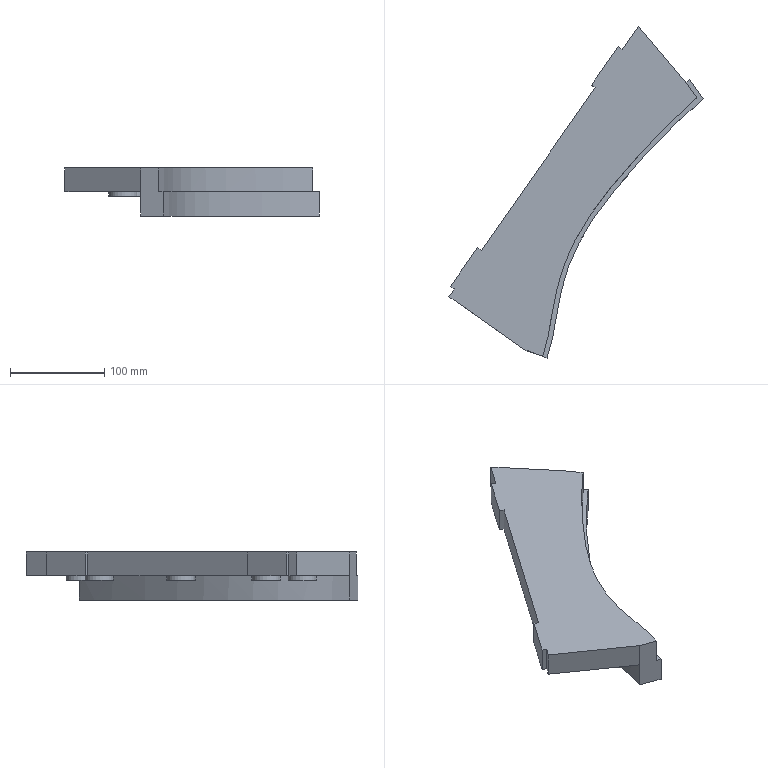Part | NX | features solid 2 | 1 solid | 31 faces | box 269.447 x 351.962 x 51 mm | volume 972041 mm3 | plane 23 | cylinder 5 | spline 3 | commonest cylinder face diameters 30 x5
STEP:
#1=CARTESIAN_POINT('',(-705.315,422.817,20.));
#2=VERTEX_POINT('',#1);
#3=CARTESIAN_POINT('',(-688.108,447.392,20.));
#4=VERTEX_POINT('',#3);
#5=CARTESIAN_POINT('',(-905.716,136.616,20.));
#6=DIRECTION('',(0.5736,0.8192,0.));
#7=VECTOR('',#6,1000.);
#8=LINE('',#5,#7);
#9=EDGE_CURVE('',#2,#4,#8,.T.);
#10=ORIENTED_EDGE('',*,*,#9,.T.);
#11=CARTESIAN_POINT('',(-637.845,387.49,20.));
#12=VERTEX_POINT('',#11);
#13=CARTESIAN_POINT('',(-624.41,371.479,20.));
#14=DIRECTION('',(-0.6428,0.766,0.));
#15=VECTOR('',#14,1000.);
#16=LINE('',#13,#15);
#17=EDGE_CURVE('',#12,#4,#16,.T.);
#18=ORIENTED_EDGE('',*,*,#17,.F.);
#19=CARTESIAN_POINT('',(-808.507,103.989,20.));
#20=VERTEX_POINT('',#19);
#21=CARTESIAN_POINT('',(-808.507,103.989,20.));
#22=CARTESIAN_POINT('',(-807.443,107.395,20.));
#23=CARTESIAN_POINT('',(-805.147,114.169,20.));
#24=CARTESIAN_POINT('',(-802.95,124.611,20.));
#25=CARTESIAN_POINT('',(-801.224,135.158,20.));
#26=CARTESIAN_POINT('',(-798.981,149.234,20.));
#27=CARTESIAN_POINT('',(-795.817,166.743,20.));
#28=CARTESIAN_POINT('',(-790.541,187.447,20.));
#29=CARTESIAN_POINT('',(-783.448,207.655,20.));
#30=CARTESIAN_POINT('',(-774.7,226.871,20.));
#31=CARTESIAN_POINT('',(-764.413,245.291,20.));
#32=CARTESIAN_POINT('',(-752.798,262.981,20.));
#33=CARTESIAN_POINT('',(-740.061,280.104,20.));
#34=CARTESIAN_POINT('',(-722.23,302.101,20.));
#35=CARTESIAN_POINT('',(-698.758,328.491,20.));
#36=CARTESIAN_POINT('',(-669.348,358.978,20.));
#37=CARTESIAN_POINT('',(-648.629,378.254,20.));
#38=CARTESIAN_POINT('',(-637.845,387.49,20.));
#39=B_SPLINE_CURVE_WITH_KNOTS('',3,(#21,#22,#23,#24,#25,#26,#27,#28,#29,#30,#31,#32,#33,#34,#35,#36,#37,#38),.UNSPECIFIED.,.F.,.F.,(4,1,1,1,1,1,1,1,1,1,1,1,1,1,1,4),(0.,0.01067,0.02134,0.03201,0.04268,0.06401,0.08535,0.1067,0.128,0.1494,0.1707,0.192,0.2134,0.2561,0.2987,0.3414),.UNSPECIFIED.);
#40=EDGE_CURVE('',#20,#12,#39,.T.);
#41=ORIENTED_EDGE('',*,*,#40,.F.);
#42=CARTESIAN_POINT('',(-889.065,160.396,20.));
#43=VERTEX_POINT('',#42);
#44=CARTESIAN_POINT('',(-845.649,129.996,20.));
#45=DIRECTION('',(-0.8192,0.5736,0.));
#46=VECTOR('',#45,1000.);
#47=LINE('',#44,#46);
#48=EDGE_CURVE('',#20,#43,#47,.T.);
#49=ORIENTED_EDGE('',*,*,#48,.T.);
#50=CARTESIAN_POINT('',(-883.329,168.587,20.));
#51=VERTEX_POINT('',#50);
#52=CARTESIAN_POINT('',(-905.716,136.616,20.));
#53=DIRECTION('',(0.5736,0.8192,0.));
#54=VECTOR('',#53,1000.);
#55=LINE('',#52,#54);
#56=EDGE_CURVE('',#43,#51,#55,.T.);
#57=ORIENTED_EDGE('',*,*,#56,.T.);
#58=CARTESIAN_POINT('',(-887.425,171.455,20.));
#59=VERTEX_POINT('',#58);
#60=CARTESIAN_POINT('',(-757.38,80.397,20.));
#61=DIRECTION('',(-0.8192,0.5736,0.));
#62=VECTOR('',#61,1000.);
#63=LINE('',#60,#62);
#64=EDGE_CURVE('',#59,#51,#63,.F.);
#65=ORIENTED_EDGE('',*,*,#64,.F.);
#66=CARTESIAN_POINT('',(-858.746,212.413,20.));
#67=VERTEX_POINT('',#66);
#68=CARTESIAN_POINT('',(-909.812,139.483,20.));
#69=DIRECTION('',(0.5736,0.8192,0.));
#70=VECTOR('',#69,1000.);
#71=LINE('',#68,#70);
#72=EDGE_CURVE('',#59,#67,#71,.T.);
#73=ORIENTED_EDGE('',*,*,#72,.T.);
#74=CARTESIAN_POINT('',(-854.65,209.545,20.));
#75=VERTEX_POINT('',#74);
#76=CARTESIAN_POINT('',(-728.701,121.354,20.));
#77=DIRECTION('',(-0.8192,0.5736,0.));
#78=VECTOR('',#77,1000.);
#79=LINE('',#76,#78);
#80=EDGE_CURVE('',#67,#75,#79,.F.);
#81=ORIENTED_EDGE('',*,*,#80,.T.);
#82=CARTESIAN_POINT('',(-733.994,381.859,20.));
#83=VERTEX_POINT('',#82);
#84=CARTESIAN_POINT('',(-905.716,136.616,20.));
#85=DIRECTION('',(0.5736,0.8192,0.));
#86=VECTOR('',#85,1000.);
#87=LINE('',#84,#86);
#88=EDGE_CURVE('',#75,#83,#87,.T.);
#89=ORIENTED_EDGE('',*,*,#88,.T.);
#90=CARTESIAN_POINT('',(-738.09,384.727,20.));
#91=VERTEX_POINT('',#90);
#92=CARTESIAN_POINT('',(-738.09,384.727,20.));
#93=DIRECTION('',(0.8192,-0.5736,0.));
#94=VECTOR('',#93,1000.);
#95=LINE('',#92,#94);
#96=EDGE_CURVE('',#91,#83,#95,.T.);
#97=ORIENTED_EDGE('',*,*,#96,.F.);
#98=CARTESIAN_POINT('',(-709.411,425.685,20.));
#99=VERTEX_POINT('',#98);
#100=CARTESIAN_POINT('',(-749.005,369.138,20.));
#101=DIRECTION('',(0.5736,0.8192,0.));
#102=VECTOR('',#101,1000.);
#103=LINE('',#100,#102);
#104=EDGE_CURVE('',#91,#99,#103,.T.);
#105=ORIENTED_EDGE('',*,*,#104,.T.);
#106=CARTESIAN_POINT('',(-709.411,425.685,20.));
#107=DIRECTION('',(0.8192,-0.5736,0.));
#108=VECTOR('',#107,1000.);
#109=LINE('',#106,#108);
#110=EDGE_CURVE('',#99,#2,#109,.T.);
#111=ORIENTED_EDGE('',*,*,#110,.T.);
#112=EDGE_LOOP('',(#10,#18,#41,#49,#57,#65,#73,#81,#89,#97,#105,#111));
#113=FACE_BOUND('',#112,.T.);
#114=CARTESIAN_POINT('',(-814.708,161.863,20.));
#115=VERTEX_POINT('',#114);
#116=CARTESIAN_POINT('',(-827.698,154.363,20.));
#117=DIRECTION('',(0.,0.,-1.));
#118=DIRECTION('',(0.866,0.5,0.));
#119=AXIS2_PLACEMENT_3D('',#116,#117,#118);
#120=CIRCLE('',#119,15.);
#121=EDGE_CURVE('',#115,#115,#120,.T.);
#122=ORIENTED_EDGE('',*,*,#121,.F.);
#123=EDGE_LOOP('',(#122));
#124=FACE_BOUND('',#123,.T.);
#125=CARTESIAN_POINT('',(-662.172,397.305,20.));
#126=VERTEX_POINT('',#125);
#127=CARTESIAN_POINT('',(-675.163,389.805,20.));
#128=DIRECTION('',(0.,0.,-1.));
#129=DIRECTION('',(0.866,0.5,0.));
#130=AXIS2_PLACEMENT_3D('',#127,#128,#129);
#131=CIRCLE('',#130,15.);
#132=EDGE_CURVE('',#126,#126,#131,.T.);
#133=ORIENTED_EDGE('',*,*,#132,.F.);
#134=EDGE_LOOP('',(#133));
#135=FACE_BOUND('',#134,.T.);
#136=CARTESIAN_POINT('',(-696.814,377.305,20.));
#137=VERTEX_POINT('',#136);
#138=CARTESIAN_POINT('',(-709.804,369.805,20.));
#139=DIRECTION('',(0.,0.,-1.));
#140=DIRECTION('',(0.866,0.5,0.));
#141=AXIS2_PLACEMENT_3D('',#138,#139,#140);
#142=CIRCLE('',#141,15.);
#143=EDGE_CURVE('',#137,#137,#142,.T.);
#144=ORIENTED_EDGE('',*,*,#143,.F.);
#145=EDGE_LOOP('',(#144));
#146=FACE_BOUND('',#145,.T.);
#147=CARTESIAN_POINT('',(-808.057,200.344,20.));
#148=VERTEX_POINT('',#147);
#149=CARTESIAN_POINT('',(-821.047,192.844,20.));
#150=DIRECTION('',(0.,0.,-1.));
#151=DIRECTION('',(0.866,0.5,0.));
#152=AXIS2_PLACEMENT_3D('',#149,#150,#151);
#153=CIRCLE('',#152,15.);
#154=EDGE_CURVE('',#148,#148,#153,.T.);
#155=ORIENTED_EDGE('',*,*,#154,.F.);
#156=EDGE_LOOP('',(#155));
#157=FACE_BOUND('',#156,.T.);
#158=CARTESIAN_POINT('',(-759.935,290.655,20.));
#159=VERTEX_POINT('',#158);
#160=CARTESIAN_POINT('',(-772.926,283.155,20.));
#161=DIRECTION('',(0.,0.,-1.));
#162=DIRECTION('',(0.866,0.5,0.));
#163=AXIS2_PLACEMENT_3D('',#160,#161,#162);
#164=CIRCLE('',#163,15.);
#165=EDGE_CURVE('',#159,#159,#164,.T.);
#166=ORIENTED_EDGE('',*,*,#165,.F.);
#167=EDGE_LOOP('',(#166));
#168=FACE_BOUND('',#167,.T.);
#169=CARTESIAN_POINT('',(-561.977,359.461,20.));
#170=DIRECTION('',(0.,0.,-1.));
#171=DIRECTION('',(-1.,0.,0.));
#172=AXIS2_PLACEMENT_3D('',#169,#170,#171);
#173=PLANE('',#172);
#174=ADVANCED_FACE('',(#113,#124,#135,#146,#157,#168),#173,.T.);
#175=CARTESIAN_POINT('',(-626.316,371.025,45.));
#176=VERTEX_POINT('',#175);
#177=CARTESIAN_POINT('',(-637.845,387.49,45.));
#178=VERTEX_POINT('',#177);
#179=CARTESIAN_POINT('',(-601.969,336.255,45.));
#180=DIRECTION('',(-0.5736,0.8192,0.));
#181=VECTOR('',#180,1000.);
#182=LINE('',#179,#181);
#183=EDGE_CURVE('',#176,#178,#182,.T.);
#184=ORIENTED_EDGE('',*,*,#183,.F.);
#185=CARTESIAN_POINT('',(-626.316,371.025,20.));
#186=VERTEX_POINT('',#185);
#187=CARTESIAN_POINT('',(-626.316,371.025,29.5));
#188=DIRECTION('',(0.,0.,1.));
#189=VECTOR('',#188,1000.);
#190=LINE('',#187,#189);
#191=EDGE_CURVE('',#176,#186,#190,.F.);
#192=ORIENTED_EDGE('',*,*,#191,.T.);
#193=CARTESIAN_POINT('',(-601.969,336.255,20.));
#194=DIRECTION('',(0.5736,-0.8192,0.));
#195=VECTOR('',#194,1000.);
#196=LINE('',#193,#195);
#197=EDGE_CURVE('',#186,#12,#196,.F.);
#198=ORIENTED_EDGE('',*,*,#197,.T.);
#199=CARTESIAN_POINT('',(-637.845,387.49,20.));
#200=DIRECTION('',(0.,0.,1.));
#201=VECTOR('',#200,1000.);
#202=LINE('',#199,#201);
#203=EDGE_CURVE('',#12,#178,#202,.T.);
#204=ORIENTED_EDGE('',*,*,#203,.T.);
#205=EDGE_LOOP('',(#184,#192,#198,#204));
#206=FACE_BOUND('',#205,.T.);
#207=CARTESIAN_POINT('',(-601.969,336.255,45.));
#208=DIRECTION('',(-0.8192,-0.5736,0.));
#209=DIRECTION('',(0.5736,-0.8192,0.));
#210=AXIS2_PLACEMENT_3D('',#207,#208,#209);
#211=PLANE('',#210);
#212=ADVANCED_FACE('',(#206),#211,.F.);
#213=CARTESIAN_POINT('',(-619.617,370.176,20.));
#214=VERTEX_POINT('',#213);
#215=CARTESIAN_POINT('',(-619.617,370.176,-6.));
#216=VERTEX_POINT('',#215);
#217=CARTESIAN_POINT('',(-619.617,370.176,45.));
#218=DIRECTION('',(0.,0.,-1.));
#219=VECTOR('',#218,1000.);
#220=LINE('',#217,#219);
#221=EDGE_CURVE('',#214,#216,#220,.T.);
#222=ORIENTED_EDGE('',*,*,#221,.F.);
#223=CARTESIAN_POINT('',(-784.99,95.429,20.));
#224=VERTEX_POINT('',#223);
#225=CARTESIAN_POINT('',(-619.617,370.176,20.));
#226=CARTESIAN_POINT('',(-620.758,369.209,20.));
#227=CARTESIAN_POINT('',(-633.301,358.48,20.));
#228=CARTESIAN_POINT('',(-656.232,336.831,20.));
#229=CARTESIAN_POINT('',(-687.219,304.143,20.));
#230=CARTESIAN_POINT('',(-716.713,270.098,20.));
#231=CARTESIAN_POINT('',(-738.935,239.768,20.));
#232=CARTESIAN_POINT('',(-753.526,213.482,20.));
#233=CARTESIAN_POINT('',(-762.494,192.807,20.));
#234=CARTESIAN_POINT('',(-769.153,171.263,20.));
#235=CARTESIAN_POINT('',(-773.765,149.208,20.));
#236=CARTESIAN_POINT('',(-776.568,130.653,20.));
#237=CARTESIAN_POINT('',(-778.83,117.715,20.));
#238=CARTESIAN_POINT('',(-780.455,110.384,20.));
#239=CARTESIAN_POINT('',(-781.918,105.166,20.));
#240=CARTESIAN_POINT('',(-783.499,100.202,20.));
#241=CARTESIAN_POINT('',(-784.493,97.02,20.));
#242=CARTESIAN_POINT('',(-784.99,95.429,20.));
#243=B_SPLINE_CURVE_WITH_KNOTS('',3,(#225,#226,#227,#228,#229,#230,#231,#232,#233,#234,#235,#236,#237,#238,#239,#240,#241,#242),.UNSPECIFIED.,.F.,.F.,(4,1,1,1,1,1,1,1,1,1,1,1,1,1,1,4),(0.,0.0136,0.1502,0.2868,0.4233,0.5599,0.6282,0.6965,0.7648,0.8331,0.9014,0.9355,0.9526,0.9697,0.9848,1.),.UNSPECIFIED.);
#244=EDGE_CURVE('',#224,#214,#243,.F.);
#245=ORIENTED_EDGE('',*,*,#244,.F.);
#246=CARTESIAN_POINT('',(-784.99,95.429,-6.));
#247=VERTEX_POINT('',#246);
#248=CARTESIAN_POINT('',(-784.99,95.429,45.));
#249=DIRECTION('',(0.,0.,-1.));
#250=VECTOR('',#249,1000.);
#251=LINE('',#248,#250);
#252=EDGE_CURVE('',#224,#247,#251,.T.);
#253=ORIENTED_EDGE('',*,*,#252,.T.);
#254=CARTESIAN_POINT('',(-619.617,370.176,-6.));
#255=CARTESIAN_POINT('',(-620.758,369.209,-6.));
#256=CARTESIAN_POINT('',(-633.301,358.48,-6.));
#257=CARTESIAN_POINT('',(-656.232,336.831,-6.));
#258=CARTESIAN_POINT('',(-687.219,304.143,-6.));
#259=CARTESIAN_POINT('',(-716.713,270.098,-6.));
#260=CARTESIAN_POINT('',(-738.935,239.768,-6.));
#261=CARTESIAN_POINT('',(-753.526,213.482,-6.));
#262=CARTESIAN_POINT('',(-762.494,192.807,-6.));
#263=CARTESIAN_POINT('',(-769.153,171.263,-6.));
#264=CARTESIAN_POINT('',(-773.765,149.208,-6.));
#265=CARTESIAN_POINT('',(-776.568,130.653,-6.));
#266=CARTESIAN_POINT('',(-778.83,117.715,-6.));
#267=CARTESIAN_POINT('',(-780.455,110.384,-6.));
#268=CARTESIAN_POINT('',(-781.918,105.166,-6.));
#269=CARTESIAN_POINT('',(-783.499,100.202,-6.));
#270=CARTESIAN_POINT('',(-784.493,97.02,-6.));
#271=CARTESIAN_POINT('',(-784.99,95.429,-6.));
#272=B_SPLINE_CURVE_WITH_KNOTS('',3,(#254,#255,#256,#257,#258,#259,#260,#261,#262,#263,#264,#265,#266,#267,#268,#269,#270,#271),.UNSPECIFIED.,.F.,.F.,(4,1,1,1,1,1,1,1,1,1,1,1,1,1,1,4),(0.,0.0136,0.1502,0.2868,0.4233,0.5599,0.6282,0.6965,0.7648,0.8331,0.9014,0.9355,0.9526,0.9697,0.9848,1.),.UNSPECIFIED.);
#273=EDGE_CURVE('',#216,#247,#272,.T.);
#274=ORIENTED_EDGE('',*,*,#273,.F.);
#275=EDGE_LOOP('',(#222,#245,#253,#274));
#276=FACE_BOUND('',#275,.T.);
#277=CARTESIAN_POINT('',(-619.617,370.176,20.));
#278=CARTESIAN_POINT('',(-619.617,370.176,-6.));
#279=CARTESIAN_POINT('',(-630.098,361.294,20.));
#280=CARTESIAN_POINT('',(-630.098,361.294,-6.));
#281=CARTESIAN_POINT('',(-650.295,342.645,20.));
#282=CARTESIAN_POINT('',(-650.295,342.645,-6.));
#283=CARTESIAN_POINT('',(-678.981,313.038,20.));
#284=CARTESIAN_POINT('',(-678.981,313.038,-6.));
#285=CARTESIAN_POINT('',(-706.428,282.292,20.));
#286=CARTESIAN_POINT('',(-706.428,282.292,-6.));
#287=CARTESIAN_POINT('',(-732.113,249.996,20.));
#288=CARTESIAN_POINT('',(-732.113,249.996,-6.));
#289=CARTESIAN_POINT('',(-750.21,220.698,20.));
#290=CARTESIAN_POINT('',(-750.21,220.698,-6.));
#291=CARTESIAN_POINT('',(-761.378,195.562,20.));
#292=CARTESIAN_POINT('',(-761.378,195.562,-6.));
#293=CARTESIAN_POINT('',(-767.84,175.972,20.));
#294=CARTESIAN_POINT('',(-767.84,175.972,-6.));
#295=CARTESIAN_POINT('',(-772.516,155.885,20.));
#296=CARTESIAN_POINT('',(-772.516,155.885,-6.));
#297=CARTESIAN_POINT('',(-775.302,138.936,20.));
#298=CARTESIAN_POINT('',(-775.302,138.936,-6.));
#299=CARTESIAN_POINT('',(-777.483,125.374,20.));
#300=CARTESIAN_POINT('',(-777.483,125.374,-6.));
#301=CARTESIAN_POINT('',(-779.274,115.224,20.));
#302=CARTESIAN_POINT('',(-779.274,115.224,-6.));
#303=CARTESIAN_POINT('',(-781.8,105.229,20.));
#304=CARTESIAN_POINT('',(-781.8,105.229,-6.));
#305=CARTESIAN_POINT('',(-783.966,98.707,20.));
#306=CARTESIAN_POINT('',(-783.966,98.707,-6.));
#307=CARTESIAN_POINT('',(-784.99,95.429,20.));
#308=CARTESIAN_POINT('',(-784.99,95.429,-6.));
#309=B_SPLINE_SURFACE_WITH_KNOTS('',3,1,((#277,#278),(#279,#280),(#281,#282),(#283,#284),(#285,#286),(#287,#288),(#289,#290),(#291,#292),(#293,#294),(#295,#296),(#297,#298),(#299,#300),(#301,#302),(#303,#304),(#305,#306),(#307,#308)),.SURF_OF_LINEAR_EXTRUSION.,.F.,.F.,.F.,(4,1,1,1,1,1,1,1,1,1,1,1,1,4),(2,2),(0.,0.125,0.25,0.375,0.5,0.625,0.6875,0.75,0.8125,0.875,0.9062,0.9375,0.9688,1.),(0.,1.),.UNSPECIFIED.);
#310=ADVANCED_FACE('',(#276),#309,.T.);
#311=ORIENTED_EDGE('',*,*,#17,.T.);
#312=CARTESIAN_POINT('',(-688.108,447.392,45.));
#313=VERTEX_POINT('',#312);
#314=CARTESIAN_POINT('',(-688.108,447.392,51.));
#315=DIRECTION('',(0.,0.,-1.));
#316=VECTOR('',#315,1000.);
#317=LINE('',#314,#316);
#318=EDGE_CURVE('',#313,#4,#317,.T.);
#319=ORIENTED_EDGE('',*,*,#318,.F.);
#320=CARTESIAN_POINT('',(-624.41,371.479,45.));
#321=DIRECTION('',(-0.6428,0.766,0.));
#322=VECTOR('',#321,1000.);
#323=LINE('',#320,#322);
#324=EDGE_CURVE('',#178,#313,#323,.T.);
#325=ORIENTED_EDGE('',*,*,#324,.F.);
#326=ORIENTED_EDGE('',*,*,#203,.F.);
#327=EDGE_LOOP('',(#311,#319,#325,#326));
#328=FACE_BOUND('',#327,.T.);
#329=CARTESIAN_POINT('',(-637.845,387.49,20.));
#330=DIRECTION('',(0.766,0.6428,0.));
#331=DIRECTION('',(-0.6428,0.766,0.));
#332=AXIS2_PLACEMENT_3D('',#329,#330,#331);
#333=PLANE('',#332);
#334=ADVANCED_FACE('',(#328),#333,.T.);
#335=ORIENTED_EDGE('',*,*,#191,.F.);
#336=CARTESIAN_POINT('',(-789.693,97.141,45.));
#337=VERTEX_POINT('',#336);
#338=CARTESIAN_POINT('',(-626.316,371.025,45.));
#339=CARTESIAN_POINT('',(-636.644,362.111,45.));
#340=CARTESIAN_POINT('',(-656.576,343.456,45.));
#341=CARTESIAN_POINT('',(-684.976,313.909,45.));
#342=CARTESIAN_POINT('',(-707.592,288.428,45.));
#343=CARTESIAN_POINT('',(-724.731,267.231,45.));
#344=CARTESIAN_POINT('',(-736.956,250.736,45.));
#345=CARTESIAN_POINT('',(-748.139,233.564,45.));
#346=CARTESIAN_POINT('',(-757.889,215.763,45.));
#347=CARTESIAN_POINT('',(-766.081,197.219,45.));
#348=CARTESIAN_POINT('',(-772.504,177.826,45.));
#349=CARTESIAN_POINT('',(-777.254,157.705,45.));
#350=CARTESIAN_POINT('',(-780.079,140.755,45.));
#351=CARTESIAN_POINT('',(-782.256,127.163,45.));
#352=CARTESIAN_POINT('',(-784.018,117.,45.));
#353=CARTESIAN_POINT('',(-786.48,106.988,45.));
#354=CARTESIAN_POINT('',(-788.665,100.433,45.));
#355=CARTESIAN_POINT('',(-789.693,97.141,45.));
#356=B_SPLINE_CURVE_WITH_KNOTS('',3,(#338,#339,#340,#341,#342,#343,#344,#345,#346,#347,#348,#349,#350,#351,#352,#353,#354,#355),.UNSPECIFIED.,.F.,.F.,(4,1,1,1,1,1,1,1,1,1,1,1,1,1,1,4),(1.377,1.418,1.459,1.5,1.521,1.541,1.562,1.582,1.603,1.623,1.643,1.664,1.674,1.684,1.695,1.705),.UNSPECIFIED.);
#357=EDGE_CURVE('',#176,#337,#356,.T.);
#358=ORIENTED_EDGE('',*,*,#357,.T.);
#359=CARTESIAN_POINT('',(-789.693,97.141,20.));
#360=VERTEX_POINT('',#359);
#361=CARTESIAN_POINT('',(-789.693,97.141,32.5));
#362=DIRECTION('',(0.,0.,1.));
#363=VECTOR('',#362,1000.);
#364=LINE('',#361,#363);
#365=EDGE_CURVE('',#360,#337,#364,.T.);
#366=ORIENTED_EDGE('',*,*,#365,.F.);
#367=CARTESIAN_POINT('',(-626.316,371.025,20.));
#368=CARTESIAN_POINT('',(-636.667,362.091,20.));
#369=CARTESIAN_POINT('',(-656.605,343.424,20.));
#370=CARTESIAN_POINT('',(-684.913,313.982,20.));
#371=CARTESIAN_POINT('',(-712.011,283.428,20.));
#372=CARTESIAN_POINT('',(-737.426,251.153,20.));
#373=CARTESIAN_POINT('',(-755.401,221.588,20.));
#374=CARTESIAN_POINT('',(-766.499,196.168,20.));
#375=CARTESIAN_POINT('',(-772.915,176.364,20.));
#376=CARTESIAN_POINT('',(-777.548,156.176,20.));
#377=CARTESIAN_POINT('',(-780.308,139.294,20.));
#378=CARTESIAN_POINT('',(-782.449,125.988,20.));
#379=CARTESIAN_POINT('',(-784.207,116.114,20.));
#380=CARTESIAN_POINT('',(-786.544,106.843,20.));
#381=CARTESIAN_POINT('',(-788.684,100.373,20.));
#382=CARTESIAN_POINT('',(-789.693,97.141,20.));
#383=B_SPLINE_CURVE_WITH_KNOTS('',3,(#367,#368,#369,#370,#371,#372,#373,#374,#375,#376,#377,#378,#379,#380,#381,#382),.UNSPECIFIED.,.F.,.F.,(4,1,1,1,1,1,1,1,1,1,1,1,1,4),(0.0137,0.1369,0.2601,0.3833,0.5065,0.6297,0.6913,0.7529,0.8145,0.8761,0.9069,0.9377,0.9685,0.9993),.UNSPECIFIED.);
#384=EDGE_CURVE('',#186,#360,#383,.T.);
#385=ORIENTED_EDGE('',*,*,#384,.F.);
#386=EDGE_LOOP('',(#335,#358,#366,#385));
#387=FACE_BOUND('',#386,.T.);
#388=CARTESIAN_POINT('',(-626.316,371.025,20.));
#389=CARTESIAN_POINT('',(-626.316,371.025,45.));
#390=CARTESIAN_POINT('',(-636.667,362.091,20.));
#391=CARTESIAN_POINT('',(-636.667,362.091,45.));
#392=CARTESIAN_POINT('',(-656.605,343.424,20.));
#393=CARTESIAN_POINT('',(-656.605,343.424,45.));
#394=CARTESIAN_POINT('',(-684.913,313.982,20.));
#395=CARTESIAN_POINT('',(-684.913,313.982,45.));
#396=CARTESIAN_POINT('',(-712.011,283.428,20.));
#397=CARTESIAN_POINT('',(-712.011,283.428,45.));
#398=CARTESIAN_POINT('',(-737.426,251.153,20.));
#399=CARTESIAN_POINT('',(-737.426,251.153,45.));
#400=CARTESIAN_POINT('',(-755.401,221.588,20.));
#401=CARTESIAN_POINT('',(-755.401,221.588,45.));
#402=CARTESIAN_POINT('',(-766.499,196.168,20.));
#403=CARTESIAN_POINT('',(-766.499,196.168,45.));
#404=CARTESIAN_POINT('',(-772.915,176.364,20.));
#405=CARTESIAN_POINT('',(-772.915,176.364,45.));
#406=CARTESIAN_POINT('',(-777.548,156.176,20.));
#407=CARTESIAN_POINT('',(-777.548,156.176,45.));
#408=CARTESIAN_POINT('',(-780.308,139.294,20.));
#409=CARTESIAN_POINT('',(-780.308,139.294,45.));
#410=CARTESIAN_POINT('',(-782.449,125.988,20.));
#411=CARTESIAN_POINT('',(-782.449,125.988,45.));
#412=CARTESIAN_POINT('',(-784.207,116.114,20.));
#413=CARTESIAN_POINT('',(-784.207,116.114,45.));
#414=CARTESIAN_POINT('',(-786.544,106.843,20.));
#415=CARTESIAN_POINT('',(-786.544,106.843,45.));
#416=CARTESIAN_POINT('',(-788.684,100.373,20.));
#417=CARTESIAN_POINT('',(-788.684,100.373,45.));
#418=CARTESIAN_POINT('',(-789.693,97.141,20.));
#419=CARTESIAN_POINT('',(-789.693,97.141,45.));
#420=B_SPLINE_SURFACE_WITH_KNOTS('',3,1,((#388,#389),(#390,#391),(#392,#393),(#394,#395),(#396,#397),(#398,#399),(#400,#401),(#402,#403),(#404,#405),(#406,#407),(#408,#409),(#410,#411),(#412,#413),(#414,#415),(#416,#417),(#418,#419)),.SURF_OF_LINEAR_EXTRUSION.,.F.,.F.,.F.,(4,1,1,1,1,1,1,1,1,1,1,1,1,4),(2,2),(0.0137,0.1369,0.2601,0.3833,0.5065,0.6297,0.6913,0.7529,0.8145,0.8761,0.9069,0.9377,0.9685,0.9993),(0.,1.),.UNSPECIFIED.);
#421=ADVANCED_FACE('',(#387),#420,.F.);
#422=ORIENTED_EDGE('',*,*,#324,.T.);
#423=CARTESIAN_POINT('',(-705.315,422.817,45.));
#424=VERTEX_POINT('',#423);
#425=CARTESIAN_POINT('',(-905.716,136.616,45.));
#426=DIRECTION('',(0.5736,0.8192,0.));
#427=VECTOR('',#426,1000.);
#428=LINE('',#425,#427);
#429=EDGE_CURVE('',#424,#313,#428,.T.);
#430=ORIENTED_EDGE('',*,*,#429,.F.);
#431=CARTESIAN_POINT('',(-709.411,425.685,45.));
#432=VERTEX_POINT('',#431);
#433=CARTESIAN_POINT('',(-661.9,392.417,45.));
#434=DIRECTION('',(0.8192,-0.5736,0.));
#435=VECTOR('',#434,1000.);
#436=LINE('',#433,#435);
#437=EDGE_CURVE('',#432,#424,#436,.T.);
#438=ORIENTED_EDGE('',*,*,#437,.F.);
#439=CARTESIAN_POINT('',(-738.09,384.727,45.));
#440=VERTEX_POINT('',#439);
#441=CARTESIAN_POINT('',(-749.005,369.138,45.));
#442=DIRECTION('',(0.5736,0.8192,0.));
#443=VECTOR('',#442,1000.);
#444=LINE('',#441,#443);
#445=EDGE_CURVE('',#440,#432,#444,.T.);
#446=ORIENTED_EDGE('',*,*,#445,.F.);
#447=CARTESIAN_POINT('',(-733.994,381.859,45.));
#448=VERTEX_POINT('',#447);
#449=CARTESIAN_POINT('',(-690.579,351.459,45.));
#450=DIRECTION('',(0.8192,-0.5736,0.));
#451=VECTOR('',#450,1000.);
#452=LINE('',#449,#451);
#453=EDGE_CURVE('',#440,#448,#452,.T.);
#454=ORIENTED_EDGE('',*,*,#453,.T.);
#455=CARTESIAN_POINT('',(-854.65,209.545,45.));
#456=VERTEX_POINT('',#455);
#457=CARTESIAN_POINT('',(-905.716,136.616,45.));
#458=DIRECTION('',(0.5736,0.8192,0.));
#459=VECTOR('',#458,1000.);
#460=LINE('',#457,#459);
#461=EDGE_CURVE('',#456,#448,#460,.T.);
#462=ORIENTED_EDGE('',*,*,#461,.F.);
#463=CARTESIAN_POINT('',(-858.746,212.413,45.));
#464=VERTEX_POINT('',#463);
#465=CARTESIAN_POINT('',(-811.235,179.145,45.));
#466=DIRECTION('',(0.8192,-0.5736,0.));
#467=VECTOR('',#466,1000.);
#468=LINE('',#465,#467);
#469=EDGE_CURVE('',#464,#456,#468,.T.);
#470=ORIENTED_EDGE('',*,*,#469,.F.);
#471=CARTESIAN_POINT('',(-887.425,171.455,45.));
#472=VERTEX_POINT('',#471);
#473=CARTESIAN_POINT('',(-909.812,139.483,45.));
#474=DIRECTION('',(0.5736,0.8192,0.));
#475=VECTOR('',#474,1000.);
#476=LINE('',#473,#475);
#477=EDGE_CURVE('',#472,#464,#476,.T.);
#478=ORIENTED_EDGE('',*,*,#477,.F.);
#479=CARTESIAN_POINT('',(-883.329,168.587,45.));
#480=VERTEX_POINT('',#479);
#481=CARTESIAN_POINT('',(-839.913,138.187,45.));
#482=DIRECTION('',(0.8192,-0.5736,0.));
#483=VECTOR('',#482,1000.);
#484=LINE('',#481,#483);
#485=EDGE_CURVE('',#472,#480,#484,.T.);
#486=ORIENTED_EDGE('',*,*,#485,.T.);
#487=CARTESIAN_POINT('',(-889.065,160.396,45.));
#488=VERTEX_POINT('',#487);
#489=CARTESIAN_POINT('',(-905.716,136.616,45.));
#490=DIRECTION('',(0.5736,0.8192,0.));
#491=VECTOR('',#490,1000.);
#492=LINE('',#489,#491);
#493=EDGE_CURVE('',#488,#480,#492,.T.);
#494=ORIENTED_EDGE('',*,*,#493,.F.);
#495=CARTESIAN_POINT('',(-808.507,103.989,45.));
#496=VERTEX_POINT('',#495);
#497=CARTESIAN_POINT('',(-845.649,129.996,45.));
#498=DIRECTION('',(-0.8192,0.5736,0.));
#499=VECTOR('',#498,1000.);
#500=LINE('',#497,#499);
#501=EDGE_CURVE('',#496,#488,#500,.T.);
#502=ORIENTED_EDGE('',*,*,#501,.F.);
#503=CARTESIAN_POINT('',(-808.507,103.989,45.));
#504=DIRECTION('',(-0.9397,0.342,0.));
#505=VECTOR('',#504,1000.);
#506=LINE('',#503,#505);
#507=EDGE_CURVE('',#337,#496,#506,.T.);
#508=ORIENTED_EDGE('',*,*,#507,.F.);
#509=ORIENTED_EDGE('',*,*,#357,.F.);
#510=ORIENTED_EDGE('',*,*,#183,.T.);
#511=EDGE_LOOP('',(#422,#430,#438,#446,#454,#462,#470,#478,#486,#494,#502,#508,#509,#510));
#512=FACE_BOUND('',#511,.T.);
#513=CARTESIAN_POINT('',(-750.849,265.384,45.));
#514=DIRECTION('',(0.,0.,1.));
#515=DIRECTION('',(1.,0.,0.));
#516=AXIS2_PLACEMENT_3D('',#513,#514,#515);
#517=PLANE('',#516);
#518=ADVANCED_FACE('',(#512),#517,.T.);
#519=ORIENTED_EDGE('',*,*,#384,.T.);
#520=CARTESIAN_POINT('',(-808.507,103.989,20.));
#521=DIRECTION('',(-0.9397,0.342,0.));
#522=VECTOR('',#521,1000.);
#523=LINE('',#520,#522);
#524=EDGE_CURVE('',#224,#360,#523,.T.);
#525=ORIENTED_EDGE('',*,*,#524,.F.);
#526=ORIENTED_EDGE('',*,*,#244,.T.);
#527=CARTESIAN_POINT('',(-634.015,390.737,20.));
#528=VERTEX_POINT('',#527);
#529=CARTESIAN_POINT('',(-619.617,370.176,20.));
#530=DIRECTION('',(0.5736,-0.8192,0.));
#531=VECTOR('',#530,1000.);
#532=LINE('',#529,#531);
#533=EDGE_CURVE('',#528,#214,#532,.T.);
#534=ORIENTED_EDGE('',*,*,#533,.F.);
#535=CARTESIAN_POINT('',(-808.507,103.989,20.));
#536=CARTESIAN_POINT('',(-808.333,104.544,20.));
#537=CARTESIAN_POINT('',(-807.867,106.034,20.));
#538=CARTESIAN_POINT('',(-806.776,109.497,20.));
#539=CARTESIAN_POINT('',(-805.771,112.695,20.));
#540=CARTESIAN_POINT('',(-804.96,115.635,20.));
#541=CARTESIAN_POINT('',(-804.266,118.437,20.));
#542=CARTESIAN_POINT('',(-803.072,124.11,20.));
#543=CARTESIAN_POINT('',(-801.552,133.064,20.));
#544=CARTESIAN_POINT('',(-799.74,144.503,20.));
#545=CARTESIAN_POINT('',(-797.693,156.521,20.));
#546=CARTESIAN_POINT('',(-794.374,172.832,20.));
#547=CARTESIAN_POINT('',(-788.796,193.527,20.));
#548=CARTESIAN_POINT('',(-779.275,217.734,20.));
#549=CARTESIAN_POINT('',(-767.447,240.431,20.));
#550=CARTESIAN_POINT('',(-753.831,261.642,20.));
#551=CARTESIAN_POINT('',(-739.131,281.358,20.));
#552=CARTESIAN_POINT('',(-723.87,299.991,20.));
#553=CARTESIAN_POINT('',(-702.884,323.901,20.));
#554=CARTESIAN_POINT('',(-675.814,352.632,20.));
#555=CARTESIAN_POINT('',(-650.572,376.631,20.));
#556=CARTESIAN_POINT('',(-636.144,388.949,20.));
#557=CARTESIAN_POINT('',(-634.015,390.737,20.));
#558=B_SPLINE_CURVE_WITH_KNOTS('',3,(#535,#536,#537,#538,#539,#540,#541,#542,#543,#544,#545,#546,#547,#548,#549,#550,#551,#552,#553,#554,#555,#556,#557),.UNSPECIFIED.,.F.,.F.,(4,1,1,1,1,1,1,1,1,1,1,1,1,1,1,1,1,1,1,1,4),(0.,0.005252,0.014,0.03149,0.04023,0.04898,0.06647,0.1015,0.1364,0.1714,0.2064,0.2764,0.3463,0.4163,0.4863,0.5562,0.6262,0.6962,0.8361,0.976,1.),.UNSPECIFIED.);
#559=EDGE_CURVE('',#528,#12,#558,.F.);
#560=ORIENTED_EDGE('',*,*,#559,.T.);
#561=ORIENTED_EDGE('',*,*,#197,.F.);
#562=EDGE_LOOP('',(#519,#525,#526,#534,#560,#561));
#563=FACE_BOUND('',#562,.T.);
#564=CARTESIAN_POINT('',(-619.617,370.176,20.));
#565=DIRECTION('',(0.,0.,-1.));
#566=DIRECTION('',(-1.,0.,0.));
#567=AXIS2_PLACEMENT_3D('',#564,#565,#566);
#568=PLANE('',#567);
#569=ADVANCED_FACE('',(#563),#568,.F.);
#570=ORIENTED_EDGE('',*,*,#501,.T.);
#571=CARTESIAN_POINT('',(-889.065,160.396,51.));
#572=DIRECTION('',(0.,0.,-1.));
#573=VECTOR('',#572,1000.);
#574=LINE('',#571,#573);
#575=EDGE_CURVE('',#488,#43,#574,.T.);
#576=ORIENTED_EDGE('',*,*,#575,.T.);
#577=ORIENTED_EDGE('',*,*,#48,.F.);
#578=CARTESIAN_POINT('',(-808.507,103.989,51.));
#579=DIRECTION('',(0.,0.,1.));
#580=VECTOR('',#579,1000.);
#581=LINE('',#578,#580);
#582=EDGE_CURVE('',#20,#496,#581,.T.);
#583=ORIENTED_EDGE('',*,*,#582,.T.);
#584=EDGE_LOOP('',(#570,#576,#577,#583));
#585=FACE_BOUND('',#584,.T.);
#586=CARTESIAN_POINT('',(-808.507,103.989,20.));
#587=DIRECTION('',(0.5736,0.8192,0.));
#588=DIRECTION('',(-0.8192,0.5736,0.));
#589=AXIS2_PLACEMENT_3D('',#586,#587,#588);
#590=PLANE('',#589);
#591=ADVANCED_FACE('',(#585),#590,.F.);
#592=ORIENTED_EDGE('',*,*,#582,.F.);
#593=CARTESIAN_POINT('',(-808.507,103.989,-6.));
#594=VERTEX_POINT('',#593);
#595=CARTESIAN_POINT('',(-808.507,103.989,45.));
#596=DIRECTION('',(0.,0.,-1.));
#597=VECTOR('',#596,1000.);
#598=LINE('',#595,#597);
#599=EDGE_CURVE('',#20,#594,#598,.T.);
#600=ORIENTED_EDGE('',*,*,#599,.T.);
#601=CARTESIAN_POINT('',(-808.507,103.989,-6.));
#602=DIRECTION('',(0.9397,-0.342,0.));
#603=VECTOR('',#602,1000.);
#604=LINE('',#601,#603);
#605=EDGE_CURVE('',#594,#247,#604,.T.);
#606=ORIENTED_EDGE('',*,*,#605,.T.);
#607=ORIENTED_EDGE('',*,*,#252,.F.);
#608=ORIENTED_EDGE('',*,*,#524,.T.);
#609=ORIENTED_EDGE('',*,*,#365,.T.);
#610=ORIENTED_EDGE('',*,*,#507,.T.);
#611=EDGE_LOOP('',(#592,#600,#606,#607,#608,#609,#610));
#612=FACE_BOUND('',#611,.T.);
#613=CARTESIAN_POINT('',(-808.507,103.989,51.));
#614=DIRECTION('',(-0.342,-0.9397,0.));
#615=DIRECTION('',(0.9397,-0.342,0.));
#616=AXIS2_PLACEMENT_3D('',#613,#614,#615);
#617=PLANE('',#616);
#618=ADVANCED_FACE('',(#612),#617,.T.);
#619=ORIENTED_EDGE('',*,*,#599,.F.);
#620=ORIENTED_EDGE('',*,*,#40,.T.);
#621=ORIENTED_EDGE('',*,*,#559,.F.);
#622=CARTESIAN_POINT('',(-634.015,390.737,-6.));
#623=VERTEX_POINT('',#622);
#624=CARTESIAN_POINT('',(-634.015,390.737,45.));
#625=DIRECTION('',(0.,0.,-1.));
#626=VECTOR('',#625,1000.);
#627=LINE('',#624,#626);
#628=EDGE_CURVE('',#528,#623,#627,.T.);
#629=ORIENTED_EDGE('',*,*,#628,.T.);
#630=CARTESIAN_POINT('',(-808.507,103.989,-6.));
#631=CARTESIAN_POINT('',(-808.333,104.544,-6.));
#632=CARTESIAN_POINT('',(-807.867,106.034,-6.));
#633=CARTESIAN_POINT('',(-806.776,109.497,-6.));
#634=CARTESIAN_POINT('',(-805.771,112.695,-6.));
#635=CARTESIAN_POINT('',(-804.96,115.635,-6.));
#636=CARTESIAN_POINT('',(-804.266,118.437,-6.));
#637=CARTESIAN_POINT('',(-803.072,124.11,-6.));
#638=CARTESIAN_POINT('',(-801.552,133.064,-6.));
#639=CARTESIAN_POINT('',(-799.74,144.503,-6.));
#640=CARTESIAN_POINT('',(-797.693,156.521,-6.));
#641=CARTESIAN_POINT('',(-794.374,172.832,-6.));
#642=CARTESIAN_POINT('',(-788.796,193.527,-6.));
#643=CARTESIAN_POINT('',(-779.275,217.734,-6.));
#644=CARTESIAN_POINT('',(-767.447,240.431,-6.));
#645=CARTESIAN_POINT('',(-753.831,261.642,-6.));
#646=CARTESIAN_POINT('',(-739.131,281.358,-6.));
#647=CARTESIAN_POINT('',(-723.87,299.991,-6.));
#648=CARTESIAN_POINT('',(-702.884,323.901,-6.));
#649=CARTESIAN_POINT('',(-675.814,352.632,-6.));
#650=CARTESIAN_POINT('',(-650.572,376.631,-6.));
#651=CARTESIAN_POINT('',(-636.144,388.949,-6.));
#652=CARTESIAN_POINT('',(-634.015,390.737,-6.));
#653=B_SPLINE_CURVE_WITH_KNOTS('',3,(#630,#631,#632,#633,#634,#635,#636,#637,#638,#639,#640,#641,#642,#643,#644,#645,#646,#647,#648,#649,#650,#651,#652),.UNSPECIFIED.,.F.,.F.,(4,1,1,1,1,1,1,1,1,1,1,1,1,1,1,1,1,1,1,1,4),(0.,0.005252,0.014,0.03149,0.04023,0.04898,0.06647,0.1015,0.1364,0.1714,0.2064,0.2764,0.3463,0.4163,0.4863,0.5562,0.6262,0.6962,0.8361,0.976,1.),.UNSPECIFIED.);
#654=EDGE_CURVE('',#594,#623,#653,.T.);
#655=ORIENTED_EDGE('',*,*,#654,.F.);
#656=EDGE_LOOP('',(#619,#620,#621,#629,#655));
#657=FACE_BOUND('',#656,.T.);
#658=CARTESIAN_POINT('',(-808.507,103.989,20.));
#659=CARTESIAN_POINT('',(-808.507,103.989,-6.));
#660=CARTESIAN_POINT('',(-807.991,105.642,20.));
#661=CARTESIAN_POINT('',(-807.991,105.642,-6.));
#662=CARTESIAN_POINT('',(-806.886,109.14,20.));
#663=CARTESIAN_POINT('',(-806.886,109.14,-6.));
#664=CARTESIAN_POINT('',(-805.545,113.441,20.));
#665=CARTESIAN_POINT('',(-805.545,113.441,-6.));
#666=CARTESIAN_POINT('',(-804.551,117.174,20.));
#667=CARTESIAN_POINT('',(-804.551,117.174,-6.));
#668=CARTESIAN_POINT('',(-803.645,121.342,20.));
#669=CARTESIAN_POINT('',(-803.645,121.342,-6.));
#670=CARTESIAN_POINT('',(-802.775,125.938,20.));
#671=CARTESIAN_POINT('',(-802.775,125.938,-6.));
#672=CARTESIAN_POINT('',(-801.679,132.325,20.));
#673=CARTESIAN_POINT('',(-801.679,132.325,-6.));
#674=CARTESIAN_POINT('',(-799.808,144.073,20.));
#675=CARTESIAN_POINT('',(-799.808,144.073,-6.));
#676=CARTESIAN_POINT('',(-796.802,162.068,20.));
#677=CARTESIAN_POINT('',(-796.802,162.068,-6.));
#678=CARTESIAN_POINT('',(-791.545,184.171,20.));
#679=CARTESIAN_POINT('',(-791.545,184.171,-6.));
#680=CARTESIAN_POINT('',(-784.119,206.139,20.));
#681=CARTESIAN_POINT('',(-784.119,206.139,-6.));
#682=CARTESIAN_POINT('',(-771.443,234.184,20.));
#683=CARTESIAN_POINT('',(-771.443,234.184,-6.));
#684=CARTESIAN_POINT('',(-751.344,266.147,20.));
#685=CARTESIAN_POINT('',(-751.344,266.147,-6.));
#686=CARTESIAN_POINT('',(-724.258,299.926,20.));
#687=CARTESIAN_POINT('',(-724.258,299.926,-6.));
#688=CARTESIAN_POINT('',(-695.94,331.532,20.));
#689=CARTESIAN_POINT('',(-695.94,331.532,-6.));
#690=CARTESIAN_POINT('',(-666.316,361.972,20.));
#691=CARTESIAN_POINT('',(-666.316,361.972,-6.));
#692=CARTESIAN_POINT('',(-645.109,381.421,20.));
#693=CARTESIAN_POINT('',(-645.109,381.421,-6.));
#694=CARTESIAN_POINT('',(-634.015,390.737,20.));
#695=CARTESIAN_POINT('',(-634.015,390.737,-6.));
#696=B_SPLINE_SURFACE_WITH_KNOTS('',3,1,((#658,#659),(#660,#661),(#662,#663),(#664,#665),(#666,#667),(#668,#669),(#670,#671),(#672,#673),(#674,#675),(#676,#677),(#678,#679),(#680,#681),(#682,#683),(#684,#685),(#686,#687),(#688,#689),(#690,#691),(#692,#693),(#694,#695)),.SURF_OF_LINEAR_EXTRUSION.,.F.,.F.,.F.,(4,1,1,1,1,1,1,1,1,1,1,1,1,1,1,1,4),(2,2),(0.,0.01562,0.03125,0.04688,0.0625,0.07812,0.09375,0.125,0.1875,0.25,0.3125,0.375,0.5,0.625,0.75,0.875,1.),(0.,1.),.UNSPECIFIED.);
#697=ADVANCED_FACE('',(#657),#696,.T.);
#698=CARTESIAN_POINT('',(-619.617,370.176,-6.));
#699=DIRECTION('',(-0.5736,0.8192,0.));
#700=VECTOR('',#699,1000.);
#701=LINE('',#698,#700);
#702=EDGE_CURVE('',#216,#623,#701,.T.);
#703=ORIENTED_EDGE('',*,*,#702,.T.);
#704=ORIENTED_EDGE('',*,*,#628,.F.);
#705=ORIENTED_EDGE('',*,*,#533,.T.);
#706=ORIENTED_EDGE('',*,*,#221,.T.);
#707=EDGE_LOOP('',(#703,#704,#705,#706));
#708=FACE_BOUND('',#707,.T.);
#709=CARTESIAN_POINT('',(-634.015,390.737,51.));
#710=DIRECTION('',(-0.8192,-0.5736,0.));
#711=DIRECTION('',(0.5736,-0.8192,0.));
#712=AXIS2_PLACEMENT_3D('',#709,#710,#711);
#713=PLANE('',#712);
#714=ADVANCED_FACE('',(#708),#713,.F.);
#715=ORIENTED_EDGE('',*,*,#654,.T.);
#716=ORIENTED_EDGE('',*,*,#702,.F.);
#717=ORIENTED_EDGE('',*,*,#273,.T.);
#718=ORIENTED_EDGE('',*,*,#605,.F.);
#719=EDGE_LOOP('',(#715,#716,#717,#718));
#720=FACE_BOUND('',#719,.T.);
#721=CARTESIAN_POINT('',(-750.849,265.384,-6.));
#722=DIRECTION('',(0.,0.,1.));
#723=DIRECTION('',(1.,0.,0.));
#724=AXIS2_PLACEMENT_3D('',#721,#722,#723);
#725=PLANE('',#724);
#726=ADVANCED_FACE('',(#720),#725,.F.);
#727=ORIENTED_EDGE('',*,*,#88,.F.);
#728=CARTESIAN_POINT('',(-854.65,209.545,51.));
#729=DIRECTION('',(0.,0.,-1.));
#730=VECTOR('',#729,1000.);
#731=LINE('',#728,#730);
#732=EDGE_CURVE('',#456,#75,#731,.T.);
#733=ORIENTED_EDGE('',*,*,#732,.F.);
#734=ORIENTED_EDGE('',*,*,#461,.T.);
#735=CARTESIAN_POINT('',(-733.994,381.859,51.));
#736=DIRECTION('',(0.,0.,-1.));
#737=VECTOR('',#736,1000.);
#738=LINE('',#735,#737);
#739=EDGE_CURVE('',#448,#83,#738,.T.);
#740=ORIENTED_EDGE('',*,*,#739,.T.);
#741=EDGE_LOOP('',(#727,#733,#734,#740));
#742=FACE_BOUND('',#741,.T.);
#743=CARTESIAN_POINT('',(-905.716,136.616,51.));
#744=DIRECTION('',(-0.8192,0.5736,0.));
#745=DIRECTION('',(-0.5736,-0.8192,0.));
#746=AXIS2_PLACEMENT_3D('',#743,#744,#745);
#747=PLANE('',#746);
#748=ADVANCED_FACE('',(#742),#747,.T.);
#749=ORIENTED_EDGE('',*,*,#9,.F.);
#750=CARTESIAN_POINT('',(-705.315,422.817,51.));
#751=DIRECTION('',(0.,0.,-1.));
#752=VECTOR('',#751,1000.);
#753=LINE('',#750,#752);
#754=EDGE_CURVE('',#424,#2,#753,.T.);
#755=ORIENTED_EDGE('',*,*,#754,.F.);
#756=ORIENTED_EDGE('',*,*,#429,.T.);
#757=ORIENTED_EDGE('',*,*,#318,.T.);
#758=EDGE_LOOP('',(#749,#755,#756,#757));
#759=FACE_BOUND('',#758,.T.);
#760=CARTESIAN_POINT('',(-905.716,136.616,51.));
#761=DIRECTION('',(-0.8192,0.5736,0.));
#762=DIRECTION('',(-0.5736,-0.8192,0.));
#763=AXIS2_PLACEMENT_3D('',#760,#761,#762);
#764=PLANE('',#763);
#765=ADVANCED_FACE('',(#759),#764,.T.);
#766=CARTESIAN_POINT('',(-883.329,168.587,51.));
#767=DIRECTION('',(0.,0.,-1.));
#768=VECTOR('',#767,1000.);
#769=LINE('',#766,#768);
#770=EDGE_CURVE('',#480,#51,#769,.T.);
#771=ORIENTED_EDGE('',*,*,#770,.T.);
#772=ORIENTED_EDGE('',*,*,#56,.F.);
#773=ORIENTED_EDGE('',*,*,#575,.F.);
#774=ORIENTED_EDGE('',*,*,#493,.T.);
#775=EDGE_LOOP('',(#771,#772,#773,#774));
#776=FACE_BOUND('',#775,.T.);
#777=CARTESIAN_POINT('',(-905.716,136.616,51.));
#778=DIRECTION('',(-0.8192,0.5736,0.));
#779=DIRECTION('',(-0.5736,-0.8192,0.));
#780=AXIS2_PLACEMENT_3D('',#777,#778,#779);
#781=PLANE('',#780);
#782=ADVANCED_FACE('',(#776),#781,.T.);
#783=ORIENTED_EDGE('',*,*,#143,.T.);
#784=EDGE_LOOP('',(#783));
#785=FACE_BOUND('',#784,.T.);
#786=CARTESIAN_POINT('',(-696.814,377.305,15.));
#787=VERTEX_POINT('',#786);
#788=CARTESIAN_POINT('',(-709.804,369.805,15.));
#789=DIRECTION('',(0.,0.,-1.));
#790=DIRECTION('',(0.866,0.5,0.));
#791=AXIS2_PLACEMENT_3D('',#788,#789,#790);
#792=CIRCLE('',#791,15.);
#793=EDGE_CURVE('',#787,#787,#792,.T.);
#794=ORIENTED_EDGE('',*,*,#793,.F.);
#795=EDGE_LOOP('',(#794));
#796=FACE_BOUND('',#795,.T.);
#797=CARTESIAN_POINT('',(-709.804,369.805,20.));
#798=DIRECTION('',(0.,0.,-1.));
#799=DIRECTION('',(-0.866,-0.5,0.));
#800=AXIS2_PLACEMENT_3D('',#797,#798,#799);
#801=CYLINDRICAL_SURFACE('',#800,15.);
#802=ADVANCED_FACE('',(#785,#796),#801,.T.);
#803=ORIENTED_EDGE('',*,*,#793,.T.);
#804=EDGE_LOOP('',(#803));
#805=FACE_BOUND('',#804,.T.);
#806=CARTESIAN_POINT('',(-709.804,369.805,15.));
#807=DIRECTION('',(0.,0.,-1.));
#808=DIRECTION('',(-0.866,-0.5,0.));
#809=AXIS2_PLACEMENT_3D('',#806,#807,#808);
#810=PLANE('',#809);
#811=ADVANCED_FACE('',(#805),#810,.T.);
#812=ORIENTED_EDGE('',*,*,#121,.T.);
#813=EDGE_LOOP('',(#812));
#814=FACE_BOUND('',#813,.T.);
#815=CARTESIAN_POINT('',(-814.708,161.863,15.));
#816=VERTEX_POINT('',#815);
#817=CARTESIAN_POINT('',(-827.698,154.363,15.));
#818=DIRECTION('',(0.,0.,-1.));
#819=DIRECTION('',(0.866,0.5,0.));
#820=AXIS2_PLACEMENT_3D('',#817,#818,#819);
#821=CIRCLE('',#820,15.);
#822=EDGE_CURVE('',#816,#816,#821,.T.);
#823=ORIENTED_EDGE('',*,*,#822,.F.);
#824=EDGE_LOOP('',(#823));
#825=FACE_BOUND('',#824,.T.);
#826=CARTESIAN_POINT('',(-827.698,154.363,20.));
#827=DIRECTION('',(0.,0.,-1.));
#828=DIRECTION('',(-0.866,-0.5,0.));
#829=AXIS2_PLACEMENT_3D('',#826,#827,#828);
#830=CYLINDRICAL_SURFACE('',#829,15.);
#831=ADVANCED_FACE('',(#814,#825),#830,.T.);
#832=ORIENTED_EDGE('',*,*,#822,.T.);
#833=EDGE_LOOP('',(#832));
#834=FACE_BOUND('',#833,.T.);
#835=CARTESIAN_POINT('',(-827.698,154.363,15.));
#836=DIRECTION('',(0.,0.,-1.));
#837=DIRECTION('',(-0.866,-0.5,0.));
#838=AXIS2_PLACEMENT_3D('',#835,#836,#837);
#839=PLANE('',#838);
#840=ADVANCED_FACE('',(#834),#839,.T.);
#841=ORIENTED_EDGE('',*,*,#154,.T.);
#842=EDGE_LOOP('',(#841));
#843=FACE_BOUND('',#842,.T.);
#844=CARTESIAN_POINT('',(-808.057,200.344,15.));
#845=VERTEX_POINT('',#844);
#846=CARTESIAN_POINT('',(-821.047,192.844,15.));
#847=DIRECTION('',(0.,0.,-1.));
#848=DIRECTION('',(0.866,0.5,0.));
#849=AXIS2_PLACEMENT_3D('',#846,#847,#848);
#850=CIRCLE('',#849,15.);
#851=EDGE_CURVE('',#845,#845,#850,.T.);
#852=ORIENTED_EDGE('',*,*,#851,.F.);
#853=EDGE_LOOP('',(#852));
#854=FACE_BOUND('',#853,.T.);
#855=CARTESIAN_POINT('',(-821.047,192.844,20.));
#856=DIRECTION('',(0.,0.,-1.));
#857=DIRECTION('',(-0.866,-0.5,0.));
#858=AXIS2_PLACEMENT_3D('',#855,#856,#857);
#859=CYLINDRICAL_SURFACE('',#858,15.);
#860=ADVANCED_FACE('',(#843,#854),#859,.T.);
#861=ORIENTED_EDGE('',*,*,#851,.T.);
#862=EDGE_LOOP('',(#861));
#863=FACE_BOUND('',#862,.T.);
#864=CARTESIAN_POINT('',(-821.047,192.844,15.));
#865=DIRECTION('',(0.,0.,-1.));
#866=DIRECTION('',(-0.866,-0.5,0.));
#867=AXIS2_PLACEMENT_3D('',#864,#865,#866);
#868=PLANE('',#867);
#869=ADVANCED_FACE('',(#863),#868,.T.);
#870=ORIENTED_EDGE('',*,*,#165,.T.);
#871=EDGE_LOOP('',(#870));
#872=FACE_BOUND('',#871,.T.);
#873=CARTESIAN_POINT('',(-759.935,290.655,15.));
#874=VERTEX_POINT('',#873);
#875=CARTESIAN_POINT('',(-772.926,283.155,15.));
#876=DIRECTION('',(0.,0.,-1.));
#877=DIRECTION('',(0.866,0.5,0.));
#878=AXIS2_PLACEMENT_3D('',#875,#876,#877);
#879=CIRCLE('',#878,15.);
#880=EDGE_CURVE('',#874,#874,#879,.T.);
#881=ORIENTED_EDGE('',*,*,#880,.F.);
#882=EDGE_LOOP('',(#881));
#883=FACE_BOUND('',#882,.T.);
#884=CARTESIAN_POINT('',(-772.926,283.155,20.));
#885=DIRECTION('',(0.,0.,-1.));
#886=DIRECTION('',(-0.866,-0.5,0.));
#887=AXIS2_PLACEMENT_3D('',#884,#885,#886);
#888=CYLINDRICAL_SURFACE('',#887,15.);
#889=ADVANCED_FACE('',(#872,#883),#888,.T.);
#890=ORIENTED_EDGE('',*,*,#880,.T.);
#891=EDGE_LOOP('',(#890));
#892=FACE_BOUND('',#891,.T.);
#893=CARTESIAN_POINT('',(-772.926,283.155,15.));
#894=DIRECTION('',(0.,0.,-1.));
#895=DIRECTION('',(-0.866,-0.5,0.));
#896=AXIS2_PLACEMENT_3D('',#893,#894,#895);
#897=PLANE('',#896);
#898=ADVANCED_FACE('',(#892),#897,.T.);
#899=ORIENTED_EDGE('',*,*,#132,.T.);
#900=EDGE_LOOP('',(#899));
#901=FACE_BOUND('',#900,.T.);
#902=CARTESIAN_POINT('',(-662.172,397.305,15.));
#903=VERTEX_POINT('',#902);
#904=CARTESIAN_POINT('',(-675.163,389.805,15.));
#905=DIRECTION('',(0.,0.,-1.));
#906=DIRECTION('',(0.866,0.5,0.));
#907=AXIS2_PLACEMENT_3D('',#904,#905,#906);
#908=CIRCLE('',#907,15.);
#909=EDGE_CURVE('',#903,#903,#908,.T.);
#910=ORIENTED_EDGE('',*,*,#909,.F.);
#911=EDGE_LOOP('',(#910));
#912=FACE_BOUND('',#911,.T.);
#913=CARTESIAN_POINT('',(-675.163,389.805,20.));
#914=DIRECTION('',(0.,0.,-1.));
#915=DIRECTION('',(-0.866,-0.5,0.));
#916=AXIS2_PLACEMENT_3D('',#913,#914,#915);
#917=CYLINDRICAL_SURFACE('',#916,15.);
#918=ADVANCED_FACE('',(#901,#912),#917,.T.);
#919=ORIENTED_EDGE('',*,*,#909,.T.);
#920=EDGE_LOOP('',(#919));
#921=FACE_BOUND('',#920,.T.);
#922=CARTESIAN_POINT('',(-675.163,389.805,15.));
#923=DIRECTION('',(0.,0.,-1.));
#924=DIRECTION('',(-0.866,-0.5,0.));
#925=AXIS2_PLACEMENT_3D('',#922,#923,#924);
#926=PLANE('',#925);
#927=ADVANCED_FACE('',(#921),#926,.T.);
#928=ORIENTED_EDGE('',*,*,#754,.T.);
#929=ORIENTED_EDGE('',*,*,#110,.F.);
#930=CARTESIAN_POINT('',(-709.411,425.685,51.));
#931=DIRECTION('',(0.,0.,-1.));
#932=VECTOR('',#931,1000.);
#933=LINE('',#930,#932);
#934=EDGE_CURVE('',#432,#99,#933,.T.);
#935=ORIENTED_EDGE('',*,*,#934,.F.);
#936=ORIENTED_EDGE('',*,*,#437,.T.);
#937=EDGE_LOOP('',(#928,#929,#935,#936));
#938=FACE_BOUND('',#937,.T.);
#939=CARTESIAN_POINT('',(-709.411,425.685,51.));
#940=DIRECTION('',(-0.5736,-0.8192,0.));
#941=DIRECTION('',(0.8192,-0.5736,0.));
#942=AXIS2_PLACEMENT_3D('',#939,#940,#941);
#943=PLANE('',#942);
#944=ADVANCED_FACE('',(#938),#943,.F.);
#945=ORIENTED_EDGE('',*,*,#739,.F.);
#946=ORIENTED_EDGE('',*,*,#453,.F.);
#947=CARTESIAN_POINT('',(-738.09,384.727,51.));
#948=DIRECTION('',(0.,0.,-1.));
#949=VECTOR('',#948,1000.);
#950=LINE('',#947,#949);
#951=EDGE_CURVE('',#440,#91,#950,.T.);
#952=ORIENTED_EDGE('',*,*,#951,.T.);
#953=ORIENTED_EDGE('',*,*,#96,.T.);
#954=EDGE_LOOP('',(#945,#946,#952,#953));
#955=FACE_BOUND('',#954,.T.);
#956=CARTESIAN_POINT('',(-738.09,384.727,51.));
#957=DIRECTION('',(-0.5736,-0.8192,0.));
#958=DIRECTION('',(0.8192,-0.5736,0.));
#959=AXIS2_PLACEMENT_3D('',#956,#957,#958);
#960=PLANE('',#959);
#961=ADVANCED_FACE('',(#955),#960,.T.);
#962=ORIENTED_EDGE('',*,*,#445,.T.);
#963=ORIENTED_EDGE('',*,*,#934,.T.);
#964=ORIENTED_EDGE('',*,*,#104,.F.);
#965=ORIENTED_EDGE('',*,*,#951,.F.);
#966=EDGE_LOOP('',(#962,#963,#964,#965));
#967=FACE_BOUND('',#966,.T.);
#968=CARTESIAN_POINT('',(-749.005,369.138,51.));
#969=DIRECTION('',(-0.8192,0.5736,0.));
#970=DIRECTION('',(-0.5736,-0.8192,0.));
#971=AXIS2_PLACEMENT_3D('',#968,#969,#970);
#972=PLANE('',#971);
#973=ADVANCED_FACE('',(#967),#972,.T.);
#974=ORIENTED_EDGE('',*,*,#732,.T.);
#975=ORIENTED_EDGE('',*,*,#80,.F.);
#976=CARTESIAN_POINT('',(-858.746,212.413,51.));
#977=DIRECTION('',(0.,0.,-1.));
#978=VECTOR('',#977,1000.);
#979=LINE('',#976,#978);
#980=EDGE_CURVE('',#464,#67,#979,.T.);
#981=ORIENTED_EDGE('',*,*,#980,.F.);
#982=ORIENTED_EDGE('',*,*,#469,.T.);
#983=EDGE_LOOP('',(#974,#975,#981,#982));
#984=FACE_BOUND('',#983,.T.);
#985=CARTESIAN_POINT('',(-858.746,212.413,51.));
#986=DIRECTION('',(-0.5736,-0.8192,0.));
#987=DIRECTION('',(0.8192,-0.5736,0.));
#988=AXIS2_PLACEMENT_3D('',#985,#986,#987);
#989=PLANE('',#988);
#990=ADVANCED_FACE('',(#984),#989,.F.);
#991=ORIENTED_EDGE('',*,*,#770,.F.);
#992=ORIENTED_EDGE('',*,*,#485,.F.);
#993=CARTESIAN_POINT('',(-887.425,171.455,51.));
#994=DIRECTION('',(0.,0.,-1.));
#995=VECTOR('',#994,1000.);
#996=LINE('',#993,#995);
#997=EDGE_CURVE('',#472,#59,#996,.T.);
#998=ORIENTED_EDGE('',*,*,#997,.T.);
#999=ORIENTED_EDGE('',*,*,#64,.T.);
#1000=EDGE_LOOP('',(#991,#992,#998,#999));
#1001=FACE_BOUND('',#1000,.T.);
#1002=CARTESIAN_POINT('',(-887.425,171.455,51.));
#1003=DIRECTION('',(-0.5736,-0.8192,0.));
#1004=DIRECTION('',(0.8192,-0.5736,0.));
#1005=AXIS2_PLACEMENT_3D('',#1002,#1003,#1004);
#1006=PLANE('',#1005);
#1007=ADVANCED_FACE('',(#1001),#1006,.T.);
#1008=ORIENTED_EDGE('',*,*,#477,.T.);
#1009=ORIENTED_EDGE('',*,*,#980,.T.);
#1010=ORIENTED_EDGE('',*,*,#72,.F.);
#1011=ORIENTED_EDGE('',*,*,#997,.F.);
#1012=EDGE_LOOP('',(#1008,#1009,#1010,#1011));
#1013=FACE_BOUND('',#1012,.T.);
#1014=CARTESIAN_POINT('',(-909.812,139.483,51.));
#1015=DIRECTION('',(-0.8192,0.5736,0.));
#1016=DIRECTION('',(-0.5736,-0.8192,0.));
#1017=AXIS2_PLACEMENT_3D('',#1014,#1015,#1016);
#1018=PLANE('',#1017);
#1019=ADVANCED_FACE('',(#1013),#1018,.T.);
#1020=CLOSED_SHELL('',(#174,#212,#310,#334,#421,#518,#569,#591,#618,#697,#714,#726,#748,#765,#782,#802,#811,#831,#840,#860,#869,#889,#898,#918,#927,#944,#961,#973,#990,#1007,#1019));
#1021=MANIFOLD_SOLID_BREP('',#1020);
#1022=(LENGTH_UNIT()NAMED_UNIT(*)SI_UNIT(.MILLI.,.METRE.));
#1023=UNCERTAINTY_MEASURE_WITH_UNIT(LENGTH_MEASURE(0.0508),#1022,'','');
#1024=(NAMED_UNIT(*)PLANE_ANGLE_UNIT()SI_UNIT($,.RADIAN.));
#1025=(NAMED_UNIT(*)SI_UNIT($,.STERADIAN.)SOLID_ANGLE_UNIT());
#1026=(GEOMETRIC_REPRESENTATION_CONTEXT(3)GLOBAL_UNCERTAINTY_ASSIGNED_CONTEXT((#1023))GLOBAL_UNIT_ASSIGNED_CONTEXT((#1022,#1024,#1025))REPRESENTATION_CONTEXT('',''));
#1027=ADVANCED_BREP_SHAPE_REPRESENTATION('',(#1021),#1026);